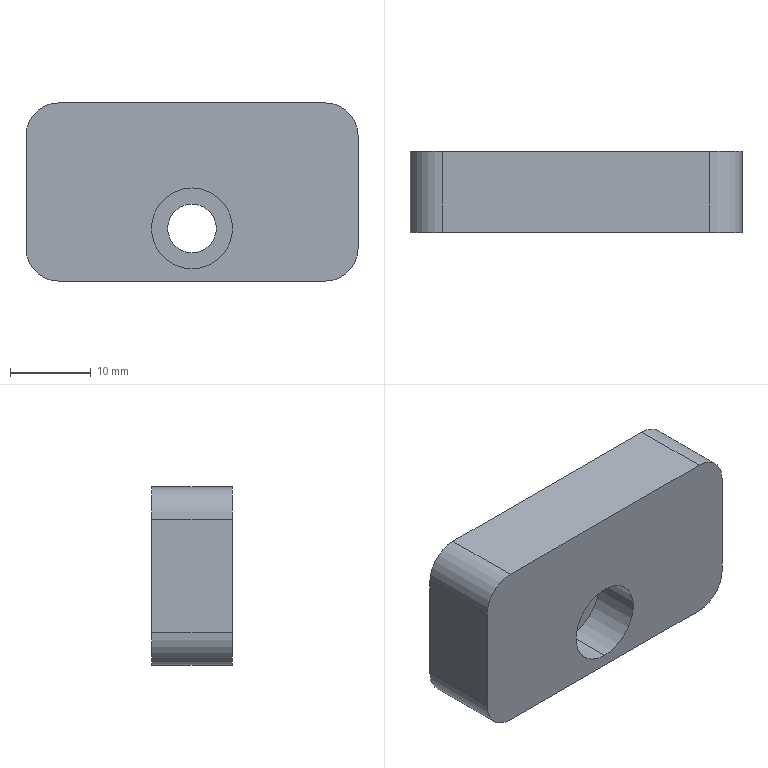Part | STEP file | 1 solid | 15 faces | box 41 x 10 x 22 mm | volume 8298 mm3 | cylinder 8 | plane 7 | commonest cylinder face diameters 8 x4 6 x2 10 x2
STEP:
#1=CARTESIAN_POINT('',(0.,0.,0.));
#2=DIRECTION('',(0.,0.,1.));
#3=DIRECTION('',(1.,0.,0.));
#4=AXIS2_PLACEMENT_3D('',#1,#2,#3);
#5=CARTESIAN_POINT('',(-118.59,-44.,195.714));
#6=VERTEX_POINT('',#5);
#7=CARTESIAN_POINT('',(-118.59,-40.,195.714));
#8=VERTEX_POINT('',#7);
#9=CARTESIAN_POINT('',(-118.59,-50.,195.714));
#10=DIRECTION('',(0.,1.,0.));
#11=VECTOR('',#10,1.);
#12=LINE('',#9,#11);
#13=CARTESIAN_POINT('',(-118.59,-50.,192.714));
#14=DIRECTION('',(0.,1.,0.));
#15=DIRECTION('',(0.,0.,1.));
#16=AXIS2_PLACEMENT_3D('',#13,#14,#15);
#17=CYLINDRICAL_SURFACE('',#16,3.);
#18=CARTESIAN_POINT('',(6.283,0.));
#19=DIRECTION('',(0.,1.));
#20=VECTOR('',#19,1.);
#21=LINE('',#18,#20);
#22=(GEOMETRIC_REPRESENTATION_CONTEXT(2)PARAMETRIC_REPRESENTATION_CONTEXT()REPRESENTATION_CONTEXT('',''));
#23=DEFINITIONAL_REPRESENTATION('',(#21),#22);
#24=PCURVE('',#17,#23);
#25=CARTESIAN_POINT('',(-118.59,-50.,192.714));
#26=DIRECTION('',(0.,1.,0.));
#27=DIRECTION('',(0.,0.,1.));
#28=AXIS2_PLACEMENT_3D('',#25,#26,#27);
#29=CYLINDRICAL_SURFACE('',#28,3.);
#30=CARTESIAN_POINT('',(0.,0.));
#31=DIRECTION('',(0.,1.));
#32=VECTOR('',#31,1.);
#33=LINE('',#30,#32);
#34=(GEOMETRIC_REPRESENTATION_CONTEXT(2)PARAMETRIC_REPRESENTATION_CONTEXT()REPRESENTATION_CONTEXT('',''));
#35=DEFINITIONAL_REPRESENTATION('',(#33),#34);
#36=PCURVE('',#29,#35);
#37=SURFACE_CURVE('',#12,(#24,#36),.PCURVE_S1.);
#38=EDGE_CURVE('',#6,#8,#37,.T.);
#39=ORIENTED_EDGE('',*,*,#38,.T.);
#40=CARTESIAN_POINT('',(-118.59,-40.,189.714));
#41=VERTEX_POINT('',#40);
#42=CARTESIAN_POINT('',(-118.59,-40.,192.714));
#43=DIRECTION('',(0.,-1.,0.));
#44=DIRECTION('',(0.,0.,-1.));
#45=AXIS2_PLACEMENT_3D('',#42,#43,#44);
#46=CIRCLE('',#45,3.);
#47=CARTESIAN_POINT('',(9.425,10.));
#48=DIRECTION('',(-1.,0.));
#49=VECTOR('',#48,1.);
#50=LINE('',#47,#49);
#51=(GEOMETRIC_REPRESENTATION_CONTEXT(2)PARAMETRIC_REPRESENTATION_CONTEXT()REPRESENTATION_CONTEXT('',''));
#52=DEFINITIONAL_REPRESENTATION('',(#50),#51);
#53=PCURVE('',#17,#52);
#54=CARTESIAN_POINT('',(-118.59,-40.,193.714));
#55=DIRECTION('',(0.,-1.,0.));
#56=DIRECTION('',(0.,0.,-1.));
#57=AXIS2_PLACEMENT_3D('',#54,#55,#56);
#58=PLANE('',#57);
#59=CARTESIAN_POINT('',(1.,0.));
#60=DIRECTION('',(1.,0.));
#61=AXIS2_PLACEMENT_2D('',#59,#60);
#62=CIRCLE('',#61,3.);
#63=(GEOMETRIC_REPRESENTATION_CONTEXT(2)PARAMETRIC_REPRESENTATION_CONTEXT()REPRESENTATION_CONTEXT('',''));
#64=DEFINITIONAL_REPRESENTATION('',(#62),#63);
#65=PCURVE('',#58,#64);
#66=SURFACE_CURVE('',#46,(#53,#65),.PCURVE_S1.);
#67=EDGE_CURVE('',#8,#41,#66,.T.);
#68=ORIENTED_EDGE('',*,*,#67,.T.);
#69=CARTESIAN_POINT('',(-118.59,-44.,189.714));
#70=VERTEX_POINT('',#69);
#71=CARTESIAN_POINT('',(-118.59,-50.,189.714));
#72=DIRECTION('',(0.,1.,0.));
#73=VECTOR('',#72,1.);
#74=LINE('',#71,#73);
#75=CARTESIAN_POINT('',(3.142,0.));
#76=DIRECTION('',(0.,1.));
#77=VECTOR('',#76,1.);
#78=LINE('',#75,#77);
#79=(GEOMETRIC_REPRESENTATION_CONTEXT(2)PARAMETRIC_REPRESENTATION_CONTEXT()REPRESENTATION_CONTEXT('',''));
#80=DEFINITIONAL_REPRESENTATION('',(#78),#79);
#81=PCURVE('',#17,#80);
#82=CARTESIAN_POINT('',(3.142,0.));
#83=DIRECTION('',(0.,1.));
#84=VECTOR('',#83,1.);
#85=LINE('',#82,#84);
#86=(GEOMETRIC_REPRESENTATION_CONTEXT(2)PARAMETRIC_REPRESENTATION_CONTEXT()REPRESENTATION_CONTEXT('',''));
#87=DEFINITIONAL_REPRESENTATION('',(#85),#86);
#88=PCURVE('',#29,#87);
#89=SURFACE_CURVE('',#74,(#81,#88),.PCURVE_S1.);
#90=EDGE_CURVE('',#70,#41,#89,.T.);
#91=ORIENTED_EDGE('',*,*,#90,.F.);
#92=CARTESIAN_POINT('',(-118.59,-44.,192.714));
#93=DIRECTION('',(0.,-1.,0.));
#94=DIRECTION('',(0.,0.,1.));
#95=AXIS2_PLACEMENT_3D('',#92,#93,#94);
#96=CIRCLE('',#95,3.);
#97=CARTESIAN_POINT('',(6.283,6.));
#98=DIRECTION('',(-1.,0.));
#99=VECTOR('',#98,1.);
#100=LINE('',#97,#99);
#101=(GEOMETRIC_REPRESENTATION_CONTEXT(2)PARAMETRIC_REPRESENTATION_CONTEXT()REPRESENTATION_CONTEXT('',''));
#102=DEFINITIONAL_REPRESENTATION('',(#100),#101);
#103=PCURVE('',#17,#102);
#104=CARTESIAN_POINT('',(-118.59,-44.,192.714));
#105=DIRECTION('',(0.,1.,0.));
#106=DIRECTION('',(0.,0.,1.));
#107=AXIS2_PLACEMENT_3D('',#104,#105,#106);
#108=PLANE('',#107);
#109=CARTESIAN_POINT('',(3.,0.));
#110=CARTESIAN_POINT('',(3.,-5.196));
#111=CARTESIAN_POINT('',(-1.5,-2.598));
#112=CARTESIAN_POINT('',(-6.,0.));
#113=CARTESIAN_POINT('',(-1.5,2.598));
#114=CARTESIAN_POINT('',(3.,5.196));
#115=CARTESIAN_POINT('',(3.,0.));
#116=(BOUNDED_CURVE()B_SPLINE_CURVE(2,(#109,#110,#111,#112,#113,#114,#115),.UNSPECIFIED.,.T.,.F.)B_SPLINE_CURVE_WITH_KNOTS((1,2,2,2,2,1),(-2.094,0.,2.094,4.189,6.283,8.378),.UNSPECIFIED.)CURVE()GEOMETRIC_REPRESENTATION_ITEM()RATIONAL_B_SPLINE_CURVE((1.,0.5,1.,0.5,1.,0.5,1.))REPRESENTATION_ITEM(''));
#117=(GEOMETRIC_REPRESENTATION_CONTEXT(2)PARAMETRIC_REPRESENTATION_CONTEXT()REPRESENTATION_CONTEXT('',''));
#118=DEFINITIONAL_REPRESENTATION('',(#116),#117);
#119=PCURVE('',#108,#118);
#120=SURFACE_CURVE('',#96,(#103,#119),.PCURVE_S1.);
#121=EDGE_CURVE('',#6,#70,#120,.T.);
#122=ORIENTED_EDGE('',*,*,#121,.F.);
#123=EDGE_LOOP('',(#39,#68,#91,#122));
#124=FACE_BOUND('',#123,.F.);
#125=ADVANCED_FACE('',(#124),#17,.F.);
#126=CARTESIAN_POINT('',(-118.59,-50.,197.714));
#127=VERTEX_POINT('',#126);
#128=CARTESIAN_POINT('',(-118.59,-44.,197.714));
#129=VERTEX_POINT('',#128);
#130=CARTESIAN_POINT('',(-118.59,-50.,197.714));
#131=DIRECTION('',(0.,1.,0.));
#132=VECTOR('',#131,1.);
#133=LINE('',#130,#132);
#134=CARTESIAN_POINT('',(-118.59,-50.,192.714));
#135=DIRECTION('',(0.,1.,0.));
#136=DIRECTION('',(0.,0.,1.));
#137=AXIS2_PLACEMENT_3D('',#134,#135,#136);
#138=CYLINDRICAL_SURFACE('',#137,5.);
#139=CARTESIAN_POINT('',(6.283,0.));
#140=DIRECTION('',(0.,1.));
#141=VECTOR('',#140,1.);
#142=LINE('',#139,#141);
#143=(GEOMETRIC_REPRESENTATION_CONTEXT(2)PARAMETRIC_REPRESENTATION_CONTEXT()REPRESENTATION_CONTEXT('',''));
#144=DEFINITIONAL_REPRESENTATION('',(#142),#143);
#145=PCURVE('',#138,#144);
#146=CARTESIAN_POINT('',(-118.59,-50.,192.714));
#147=DIRECTION('',(0.,1.,0.));
#148=DIRECTION('',(0.,0.,1.));
#149=AXIS2_PLACEMENT_3D('',#146,#147,#148);
#150=CYLINDRICAL_SURFACE('',#149,5.);
#151=CARTESIAN_POINT('',(0.,0.));
#152=DIRECTION('',(0.,1.));
#153=VECTOR('',#152,1.);
#154=LINE('',#151,#153);
#155=(GEOMETRIC_REPRESENTATION_CONTEXT(2)PARAMETRIC_REPRESENTATION_CONTEXT()REPRESENTATION_CONTEXT('',''));
#156=DEFINITIONAL_REPRESENTATION('',(#154),#155);
#157=PCURVE('',#150,#156);
#158=SURFACE_CURVE('',#133,(#145,#157),.PCURVE_S1.);
#159=EDGE_CURVE('',#127,#129,#158,.T.);
#160=ORIENTED_EDGE('',*,*,#159,.T.);
#161=CARTESIAN_POINT('',(-118.59,-44.,187.714));
#162=VERTEX_POINT('',#161);
#163=CARTESIAN_POINT('',(-118.59,-44.,192.714));
#164=DIRECTION('',(0.,-1.,0.));
#165=DIRECTION('',(0.,0.,-1.));
#166=AXIS2_PLACEMENT_3D('',#163,#164,#165);
#167=CIRCLE('',#166,5.);
#168=CARTESIAN_POINT('',(9.425,6.));
#169=DIRECTION('',(-1.,0.));
#170=VECTOR('',#169,1.);
#171=LINE('',#168,#170);
#172=(GEOMETRIC_REPRESENTATION_CONTEXT(2)PARAMETRIC_REPRESENTATION_CONTEXT()REPRESENTATION_CONTEXT('',''));
#173=DEFINITIONAL_REPRESENTATION('',(#171),#172);
#174=PCURVE('',#138,#173);
#175=CARTESIAN_POINT('',(-5.,0.));
#176=CARTESIAN_POINT('',(-5.,8.66));
#177=CARTESIAN_POINT('',(2.5,4.33));
#178=CARTESIAN_POINT('',(10.,0.));
#179=CARTESIAN_POINT('',(2.5,-4.33));
#180=CARTESIAN_POINT('',(-5.,-8.66));
#181=CARTESIAN_POINT('',(-5.,0.));
#182=(BOUNDED_CURVE()B_SPLINE_CURVE(2,(#175,#176,#177,#178,#179,#180,#181),.UNSPECIFIED.,.T.,.F.)B_SPLINE_CURVE_WITH_KNOTS((1,2,2,2,2,1),(-2.094,0.,2.094,4.189,6.283,8.378),.UNSPECIFIED.)CURVE()GEOMETRIC_REPRESENTATION_ITEM()RATIONAL_B_SPLINE_CURVE((1.,0.5,1.,0.5,1.,0.5,1.))REPRESENTATION_ITEM(''));
#183=(GEOMETRIC_REPRESENTATION_CONTEXT(2)PARAMETRIC_REPRESENTATION_CONTEXT()REPRESENTATION_CONTEXT('',''));
#184=DEFINITIONAL_REPRESENTATION('',(#182),#183);
#185=PCURVE('',#108,#184);
#186=SURFACE_CURVE('',#167,(#174,#185),.PCURVE_S1.);
#187=EDGE_CURVE('',#129,#162,#186,.T.);
#188=ORIENTED_EDGE('',*,*,#187,.T.);
#189=CARTESIAN_POINT('',(-118.59,-50.,187.714));
#190=VERTEX_POINT('',#189);
#191=CARTESIAN_POINT('',(-118.59,-50.,187.714));
#192=DIRECTION('',(0.,1.,0.));
#193=VECTOR('',#192,1.);
#194=LINE('',#191,#193);
#195=CARTESIAN_POINT('',(3.142,0.));
#196=DIRECTION('',(0.,1.));
#197=VECTOR('',#196,1.);
#198=LINE('',#195,#197);
#199=(GEOMETRIC_REPRESENTATION_CONTEXT(2)PARAMETRIC_REPRESENTATION_CONTEXT()REPRESENTATION_CONTEXT('',''));
#200=DEFINITIONAL_REPRESENTATION('',(#198),#199);
#201=PCURVE('',#138,#200);
#202=CARTESIAN_POINT('',(3.142,0.));
#203=DIRECTION('',(0.,1.));
#204=VECTOR('',#203,1.);
#205=LINE('',#202,#204);
#206=(GEOMETRIC_REPRESENTATION_CONTEXT(2)PARAMETRIC_REPRESENTATION_CONTEXT()REPRESENTATION_CONTEXT('',''));
#207=DEFINITIONAL_REPRESENTATION('',(#205),#206);
#208=PCURVE('',#150,#207);
#209=SURFACE_CURVE('',#194,(#201,#208),.PCURVE_S1.);
#210=EDGE_CURVE('',#190,#162,#209,.T.);
#211=ORIENTED_EDGE('',*,*,#210,.F.);
#212=CARTESIAN_POINT('',(-118.59,-50.,192.714));
#213=DIRECTION('',(0.,1.,0.));
#214=DIRECTION('',(0.,0.,1.));
#215=AXIS2_PLACEMENT_3D('',#212,#213,#214);
#216=CIRCLE('',#215,5.);
#217=CARTESIAN_POINT('',(0.,0.));
#218=DIRECTION('',(1.,0.));
#219=VECTOR('',#218,1.);
#220=LINE('',#217,#219);
#221=(GEOMETRIC_REPRESENTATION_CONTEXT(2)PARAMETRIC_REPRESENTATION_CONTEXT()REPRESENTATION_CONTEXT('',''));
#222=DEFINITIONAL_REPRESENTATION('',(#220),#221);
#223=PCURVE('',#138,#222);
#224=CARTESIAN_POINT('',(-118.59,-50.,189.963));
#225=DIRECTION('',(0.,-1.,0.));
#226=DIRECTION('',(0.,0.,-1.));
#227=AXIS2_PLACEMENT_3D('',#224,#225,#226);
#228=PLANE('',#227);
#229=CARTESIAN_POINT('',(-7.751,0.));
#230=CARTESIAN_POINT('',(-7.751,8.66));
#231=CARTESIAN_POINT('',(-0.2512,4.33));
#232=CARTESIAN_POINT('',(7.249,0.));
#233=CARTESIAN_POINT('',(-0.2512,-4.33));
#234=CARTESIAN_POINT('',(-7.751,-8.66));
#235=CARTESIAN_POINT('',(-7.751,0.));
#236=(BOUNDED_CURVE()B_SPLINE_CURVE(2,(#229,#230,#231,#232,#233,#234,#235),.UNSPECIFIED.,.T.,.F.)B_SPLINE_CURVE_WITH_KNOTS((1,2,2,2,2,1),(-2.094,0.,2.094,4.189,6.283,8.378),.UNSPECIFIED.)CURVE()GEOMETRIC_REPRESENTATION_ITEM()RATIONAL_B_SPLINE_CURVE((1.,0.5,1.,0.5,1.,0.5,1.))REPRESENTATION_ITEM(''));
#237=(GEOMETRIC_REPRESENTATION_CONTEXT(2)PARAMETRIC_REPRESENTATION_CONTEXT()REPRESENTATION_CONTEXT('',''));
#238=DEFINITIONAL_REPRESENTATION('',(#236),#237);
#239=PCURVE('',#228,#238);
#240=SURFACE_CURVE('',#216,(#223,#239),.PCURVE_S1.);
#241=EDGE_CURVE('',#190,#127,#240,.T.);
#242=ORIENTED_EDGE('',*,*,#241,.T.);
#243=EDGE_LOOP('',(#160,#188,#211,#242));
#244=FACE_BOUND('',#243,.F.);
#245=ADVANCED_FACE('',(#244),#138,.F.);
#246=CARTESIAN_POINT('',(-102.09,-50.,208.214));
#247=VERTEX_POINT('',#246);
#248=CARTESIAN_POINT('',(-135.09,-50.,208.214));
#249=VERTEX_POINT('',#248);
#250=CARTESIAN_POINT('',(-118.59,-50.,208.214));
#251=DIRECTION('',(-1.,0.,0.));
#252=VECTOR('',#251,1.);
#253=LINE('',#250,#252);
#254=CARTESIAN_POINT('',(-18.251,0.));
#255=DIRECTION('',(0.,-1.));
#256=VECTOR('',#255,1.);
#257=LINE('',#254,#256);
#258=(GEOMETRIC_REPRESENTATION_CONTEXT(2)PARAMETRIC_REPRESENTATION_CONTEXT()REPRESENTATION_CONTEXT('',''));
#259=DEFINITIONAL_REPRESENTATION('',(#257),#258);
#260=PCURVE('',#228,#259);
#261=CARTESIAN_POINT('',(-98.09,-40.,208.214));
#262=DIRECTION('',(0.,0.,1.));
#263=DIRECTION('',(1.,0.,0.));
#264=AXIS2_PLACEMENT_3D('',#261,#262,#263);
#265=PLANE('',#264);
#266=CARTESIAN_POINT('',(-20.5,-10.));
#267=DIRECTION('',(-1.,0.));
#268=VECTOR('',#267,1.);
#269=LINE('',#266,#268);
#270=(GEOMETRIC_REPRESENTATION_CONTEXT(2)PARAMETRIC_REPRESENTATION_CONTEXT()REPRESENTATION_CONTEXT('',''));
#271=DEFINITIONAL_REPRESENTATION('',(#269),#270);
#272=PCURVE('',#265,#271);
#273=SURFACE_CURVE('',#253,(#260,#272),.PCURVE_S1.);
#274=EDGE_CURVE('',#247,#249,#273,.T.);
#275=ORIENTED_EDGE('',*,*,#274,.T.);
#276=CARTESIAN_POINT('',(-139.09,-50.,204.214));
#277=VERTEX_POINT('',#276);
#278=CARTESIAN_POINT('',(-135.09,-50.,204.214));
#279=DIRECTION('',(0.,-1.,0.));
#280=DIRECTION('',(0.,0.,-1.));
#281=AXIS2_PLACEMENT_3D('',#278,#279,#280);
#282=CIRCLE('',#281,4.);
#283=CARTESIAN_POINT('',(-14.251,-16.5));
#284=DIRECTION('',(1.,0.));
#285=AXIS2_PLACEMENT_2D('',#283,#284);
#286=CIRCLE('',#285,4.);
#287=(GEOMETRIC_REPRESENTATION_CONTEXT(2)PARAMETRIC_REPRESENTATION_CONTEXT()REPRESENTATION_CONTEXT('',''));
#288=DEFINITIONAL_REPRESENTATION('',(#286),#287);
#289=PCURVE('',#228,#288);
#290=CARTESIAN_POINT('',(-135.09,-50.,204.214));
#291=DIRECTION('',(0.,-1.,0.));
#292=DIRECTION('',(0.,0.,-1.));
#293=AXIS2_PLACEMENT_3D('',#290,#291,#292);
#294=CYLINDRICAL_SURFACE('',#293,4.);
#295=CARTESIAN_POINT('',(0.,0.));
#296=DIRECTION('',(1.,0.));
#297=VECTOR('',#296,1.);
#298=LINE('',#295,#297);
#299=(GEOMETRIC_REPRESENTATION_CONTEXT(2)PARAMETRIC_REPRESENTATION_CONTEXT()REPRESENTATION_CONTEXT('',''));
#300=DEFINITIONAL_REPRESENTATION('',(#298),#299);
#301=PCURVE('',#294,#300);
#302=SURFACE_CURVE('',#282,(#289,#301),.PCURVE_S1.);
#303=EDGE_CURVE('',#249,#277,#302,.T.);
#304=ORIENTED_EDGE('',*,*,#303,.T.);
#305=CARTESIAN_POINT('',(-139.09,-50.,190.214));
#306=VERTEX_POINT('',#305);
#307=CARTESIAN_POINT('',(-139.09,-50.,189.963));
#308=DIRECTION('',(0.,0.,1.));
#309=VECTOR('',#308,1.);
#310=LINE('',#307,#309);
#311=CARTESIAN_POINT('',(0.,-20.5));
#312=DIRECTION('',(-1.,0.));
#313=VECTOR('',#312,1.);
#314=LINE('',#311,#313);
#315=(GEOMETRIC_REPRESENTATION_CONTEXT(2)PARAMETRIC_REPRESENTATION_CONTEXT()REPRESENTATION_CONTEXT('',''));
#316=DEFINITIONAL_REPRESENTATION('',(#314),#315);
#317=PCURVE('',#228,#316);
#318=CARTESIAN_POINT('',(-139.09,-50.,202.465));
#319=DIRECTION('',(1.,0.,0.));
#320=DIRECTION('',(0.,0.,-1.));
#321=AXIS2_PLACEMENT_3D('',#318,#319,#320);
#322=PLANE('',#321);
#323=CARTESIAN_POINT('',(12.502,0.));
#324=DIRECTION('',(-1.,0.));
#325=VECTOR('',#324,1.);
#326=LINE('',#323,#325);
#327=(GEOMETRIC_REPRESENTATION_CONTEXT(2)PARAMETRIC_REPRESENTATION_CONTEXT()REPRESENTATION_CONTEXT('',''));
#328=DEFINITIONAL_REPRESENTATION('',(#326),#327);
#329=PCURVE('',#322,#328);
#330=SURFACE_CURVE('',#310,(#317,#329),.PCURVE_S1.);
#331=EDGE_CURVE('',#306,#277,#330,.T.);
#332=ORIENTED_EDGE('',*,*,#331,.F.);
#333=CARTESIAN_POINT('',(-135.09,-50.,186.214));
#334=VERTEX_POINT('',#333);
#335=CARTESIAN_POINT('',(-135.09,-50.,190.214));
#336=DIRECTION('',(0.,-1.,0.));
#337=DIRECTION('',(0.,0.,-1.));
#338=AXIS2_PLACEMENT_3D('',#335,#336,#337);
#339=CIRCLE('',#338,4.);
#340=CARTESIAN_POINT('',(-0.2512,-16.5));
#341=DIRECTION('',(1.,0.));
#342=AXIS2_PLACEMENT_2D('',#340,#341);
#343=CIRCLE('',#342,4.);
#344=(GEOMETRIC_REPRESENTATION_CONTEXT(2)PARAMETRIC_REPRESENTATION_CONTEXT()REPRESENTATION_CONTEXT('',''));
#345=DEFINITIONAL_REPRESENTATION('',(#343),#344);
#346=PCURVE('',#228,#345);
#347=CARTESIAN_POINT('',(-135.09,-50.,190.214));
#348=DIRECTION('',(0.,-1.,0.));
#349=DIRECTION('',(0.,0.,-1.));
#350=AXIS2_PLACEMENT_3D('',#347,#348,#349);
#351=CYLINDRICAL_SURFACE('',#350,4.);
#352=CARTESIAN_POINT('',(0.,0.));
#353=DIRECTION('',(1.,0.));
#354=VECTOR('',#353,1.);
#355=LINE('',#352,#354);
#356=(GEOMETRIC_REPRESENTATION_CONTEXT(2)PARAMETRIC_REPRESENTATION_CONTEXT()REPRESENTATION_CONTEXT('',''));
#357=DEFINITIONAL_REPRESENTATION('',(#355),#356);
#358=PCURVE('',#351,#357);
#359=SURFACE_CURVE('',#339,(#346,#358),.PCURVE_S1.);
#360=EDGE_CURVE('',#306,#334,#359,.T.);
#361=ORIENTED_EDGE('',*,*,#360,.T.);
#362=CARTESIAN_POINT('',(-102.09,-50.,186.214));
#363=VERTEX_POINT('',#362);
#364=CARTESIAN_POINT('',(-118.59,-50.,186.214));
#365=DIRECTION('',(-1.,0.,0.));
#366=VECTOR('',#365,1.);
#367=LINE('',#364,#366);
#368=CARTESIAN_POINT('',(3.749,0.));
#369=DIRECTION('',(0.,-1.));
#370=VECTOR('',#369,1.);
#371=LINE('',#368,#370);
#372=(GEOMETRIC_REPRESENTATION_CONTEXT(2)PARAMETRIC_REPRESENTATION_CONTEXT()REPRESENTATION_CONTEXT('',''));
#373=DEFINITIONAL_REPRESENTATION('',(#371),#372);
#374=PCURVE('',#228,#373);
#375=CARTESIAN_POINT('',(-98.09,-40.,186.214));
#376=DIRECTION('',(0.,0.,1.));
#377=DIRECTION('',(1.,0.,0.));
#378=AXIS2_PLACEMENT_3D('',#375,#376,#377);
#379=PLANE('',#378);
#380=CARTESIAN_POINT('',(-20.5,-10.));
#381=DIRECTION('',(-1.,0.));
#382=VECTOR('',#381,1.);
#383=LINE('',#380,#382);
#384=(GEOMETRIC_REPRESENTATION_CONTEXT(2)PARAMETRIC_REPRESENTATION_CONTEXT()REPRESENTATION_CONTEXT('',''));
#385=DEFINITIONAL_REPRESENTATION('',(#383),#384);
#386=PCURVE('',#379,#385);
#387=SURFACE_CURVE('',#367,(#374,#386),.PCURVE_S1.);
#388=EDGE_CURVE('',#363,#334,#387,.T.);
#389=ORIENTED_EDGE('',*,*,#388,.F.);
#390=CARTESIAN_POINT('',(-98.09,-50.,190.214));
#391=VERTEX_POINT('',#390);
#392=CARTESIAN_POINT('',(-102.09,-50.,190.214));
#393=DIRECTION('',(0.,-1.,0.));
#394=DIRECTION('',(0.,0.,-1.));
#395=AXIS2_PLACEMENT_3D('',#392,#393,#394);
#396=CIRCLE('',#395,4.);
#397=CARTESIAN_POINT('',(-0.2512,16.5));
#398=DIRECTION('',(1.,0.));
#399=AXIS2_PLACEMENT_2D('',#397,#398);
#400=CIRCLE('',#399,4.);
#401=(GEOMETRIC_REPRESENTATION_CONTEXT(2)PARAMETRIC_REPRESENTATION_CONTEXT()REPRESENTATION_CONTEXT('',''));
#402=DEFINITIONAL_REPRESENTATION('',(#400),#401);
#403=PCURVE('',#228,#402);
#404=CARTESIAN_POINT('',(-102.09,-40.,190.214));
#405=DIRECTION('',(0.,1.,0.));
#406=DIRECTION('',(0.,0.,1.));
#407=AXIS2_PLACEMENT_3D('',#404,#405,#406);
#408=CYLINDRICAL_SURFACE('',#407,4.);
#409=CARTESIAN_POINT('',(3.142,-10.));
#410=DIRECTION('',(-1.,0.));
#411=VECTOR('',#410,1.);
#412=LINE('',#409,#411);
#413=(GEOMETRIC_REPRESENTATION_CONTEXT(2)PARAMETRIC_REPRESENTATION_CONTEXT()REPRESENTATION_CONTEXT('',''));
#414=DEFINITIONAL_REPRESENTATION('',(#412),#413);
#415=PCURVE('',#408,#414);
#416=SURFACE_CURVE('',#396,(#403,#415),.PCURVE_S1.);
#417=EDGE_CURVE('',#363,#391,#416,.T.);
#418=ORIENTED_EDGE('',*,*,#417,.T.);
#419=CARTESIAN_POINT('',(-98.09,-50.,204.214));
#420=VERTEX_POINT('',#419);
#421=CARTESIAN_POINT('',(-98.09,-50.,189.963));
#422=DIRECTION('',(0.,0.,1.));
#423=VECTOR('',#422,1.);
#424=LINE('',#421,#423);
#425=CARTESIAN_POINT('',(0.,20.5));
#426=DIRECTION('',(-1.,0.));
#427=VECTOR('',#426,1.);
#428=LINE('',#425,#427);
#429=(GEOMETRIC_REPRESENTATION_CONTEXT(2)PARAMETRIC_REPRESENTATION_CONTEXT()REPRESENTATION_CONTEXT('',''));
#430=DEFINITIONAL_REPRESENTATION('',(#428),#429);
#431=PCURVE('',#228,#430);
#432=CARTESIAN_POINT('',(-98.09,-50.,202.465));
#433=DIRECTION('',(1.,0.,0.));
#434=DIRECTION('',(0.,0.,-1.));
#435=AXIS2_PLACEMENT_3D('',#432,#433,#434);
#436=PLANE('',#435);
#437=CARTESIAN_POINT('',(12.502,0.));
#438=DIRECTION('',(-1.,0.));
#439=VECTOR('',#438,1.);
#440=LINE('',#437,#439);
#441=(GEOMETRIC_REPRESENTATION_CONTEXT(2)PARAMETRIC_REPRESENTATION_CONTEXT()REPRESENTATION_CONTEXT('',''));
#442=DEFINITIONAL_REPRESENTATION('',(#440),#441);
#443=PCURVE('',#436,#442);
#444=SURFACE_CURVE('',#424,(#431,#443),.PCURVE_S1.);
#445=EDGE_CURVE('',#391,#420,#444,.T.);
#446=ORIENTED_EDGE('',*,*,#445,.T.);
#447=CARTESIAN_POINT('',(-102.09,-50.,204.214));
#448=DIRECTION('',(0.,-1.,0.));
#449=DIRECTION('',(0.,0.,-1.));
#450=AXIS2_PLACEMENT_3D('',#447,#448,#449);
#451=CIRCLE('',#450,4.);
#452=CARTESIAN_POINT('',(-14.251,16.5));
#453=DIRECTION('',(1.,0.));
#454=AXIS2_PLACEMENT_2D('',#452,#453);
#455=CIRCLE('',#454,4.);
#456=(GEOMETRIC_REPRESENTATION_CONTEXT(2)PARAMETRIC_REPRESENTATION_CONTEXT()REPRESENTATION_CONTEXT('',''));
#457=DEFINITIONAL_REPRESENTATION('',(#455),#456);
#458=PCURVE('',#228,#457);
#459=CARTESIAN_POINT('',(-102.09,-40.,204.214));
#460=DIRECTION('',(0.,1.,0.));
#461=DIRECTION('',(0.,0.,1.));
#462=AXIS2_PLACEMENT_3D('',#459,#460,#461);
#463=CYLINDRICAL_SURFACE('',#462,4.);
#464=CARTESIAN_POINT('',(3.142,-10.));
#465=DIRECTION('',(-1.,0.));
#466=VECTOR('',#465,1.);
#467=LINE('',#464,#466);
#468=(GEOMETRIC_REPRESENTATION_CONTEXT(2)PARAMETRIC_REPRESENTATION_CONTEXT()REPRESENTATION_CONTEXT('',''));
#469=DEFINITIONAL_REPRESENTATION('',(#467),#468);
#470=PCURVE('',#463,#469);
#471=SURFACE_CURVE('',#451,(#458,#470),.PCURVE_S1.);
#472=EDGE_CURVE('',#420,#247,#471,.T.);
#473=ORIENTED_EDGE('',*,*,#472,.T.);
#474=EDGE_LOOP('',(#275,#304,#332,#361,#389,#418,#446,#473));
#475=FACE_BOUND('',#474,.T.);
#476=CARTESIAN_POINT('',(-118.59,-50.,192.714));
#477=DIRECTION('',(0.,1.,0.));
#478=DIRECTION('',(0.,0.,1.));
#479=AXIS2_PLACEMENT_3D('',#476,#477,#478);
#480=CIRCLE('',#479,5.);
#481=CARTESIAN_POINT('',(-7.751,0.));
#482=CARTESIAN_POINT('',(-7.751,8.66));
#483=CARTESIAN_POINT('',(-0.2512,4.33));
#484=CARTESIAN_POINT('',(7.249,0.));
#485=CARTESIAN_POINT('',(-0.2512,-4.33));
#486=CARTESIAN_POINT('',(-7.751,-8.66));
#487=CARTESIAN_POINT('',(-7.751,0.));
#488=(BOUNDED_CURVE()B_SPLINE_CURVE(2,(#481,#482,#483,#484,#485,#486,#487),.UNSPECIFIED.,.T.,.F.)B_SPLINE_CURVE_WITH_KNOTS((1,2,2,2,2,1),(-2.094,0.,2.094,4.189,6.283,8.378),.UNSPECIFIED.)CURVE()GEOMETRIC_REPRESENTATION_ITEM()RATIONAL_B_SPLINE_CURVE((1.,0.5,1.,0.5,1.,0.5,1.))REPRESENTATION_ITEM(''));
#489=(GEOMETRIC_REPRESENTATION_CONTEXT(2)PARAMETRIC_REPRESENTATION_CONTEXT()REPRESENTATION_CONTEXT('',''));
#490=DEFINITIONAL_REPRESENTATION('',(#488),#489);
#491=PCURVE('',#228,#490);
#492=CARTESIAN_POINT('',(0.,0.));
#493=DIRECTION('',(1.,0.));
#494=VECTOR('',#493,1.);
#495=LINE('',#492,#494);
#496=(GEOMETRIC_REPRESENTATION_CONTEXT(2)PARAMETRIC_REPRESENTATION_CONTEXT()REPRESENTATION_CONTEXT('',''));
#497=DEFINITIONAL_REPRESENTATION('',(#495),#496);
#498=PCURVE('',#150,#497);
#499=SURFACE_CURVE('',#480,(#491,#498),.PCURVE_S1.);
#500=EDGE_CURVE('',#127,#190,#499,.T.);
#501=ORIENTED_EDGE('',*,*,#500,.T.);
#502=ORIENTED_EDGE('',*,*,#241,.T.);
#503=EDGE_LOOP('',(#501,#502));
#504=FACE_BOUND('',#503,.T.);
#505=ADVANCED_FACE('',(#475,#504),#228,.T.);
#506=CARTESIAN_POINT('',(-102.09,-40.,208.214));
#507=VERTEX_POINT('',#506);
#508=CARTESIAN_POINT('',(-135.09,-40.,208.214));
#509=VERTEX_POINT('',#508);
#510=CARTESIAN_POINT('',(-118.59,-40.,208.214));
#511=DIRECTION('',(-1.,0.,0.));
#512=VECTOR('',#511,1.);
#513=LINE('',#510,#512);
#514=CARTESIAN_POINT('',(-20.5,0.));
#515=DIRECTION('',(-1.,0.));
#516=VECTOR('',#515,1.);
#517=LINE('',#514,#516);
#518=(GEOMETRIC_REPRESENTATION_CONTEXT(2)PARAMETRIC_REPRESENTATION_CONTEXT()REPRESENTATION_CONTEXT('',''));
#519=DEFINITIONAL_REPRESENTATION('',(#517),#518);
#520=PCURVE('',#265,#519);
#521=CARTESIAN_POINT('',(-14.5,0.));
#522=DIRECTION('',(0.,-1.));
#523=VECTOR('',#522,1.);
#524=LINE('',#521,#523);
#525=(GEOMETRIC_REPRESENTATION_CONTEXT(2)PARAMETRIC_REPRESENTATION_CONTEXT()REPRESENTATION_CONTEXT('',''));
#526=DEFINITIONAL_REPRESENTATION('',(#524),#525);
#527=PCURVE('',#58,#526);
#528=SURFACE_CURVE('',#513,(#520,#527),.PCURVE_S1.);
#529=EDGE_CURVE('',#507,#509,#528,.T.);
#530=ORIENTED_EDGE('',*,*,#529,.T.);
#531=CARTESIAN_POINT('',(-135.09,-50.,208.214));
#532=DIRECTION('',(0.,-1.,0.));
#533=VECTOR('',#532,1.);
#534=LINE('',#531,#533);
#535=CARTESIAN_POINT('',(-37.,-10.));
#536=DIRECTION('',(0.,-1.));
#537=VECTOR('',#536,1.);
#538=LINE('',#535,#537);
#539=(GEOMETRIC_REPRESENTATION_CONTEXT(2)PARAMETRIC_REPRESENTATION_CONTEXT()REPRESENTATION_CONTEXT('',''));
#540=DEFINITIONAL_REPRESENTATION('',(#538),#539);
#541=PCURVE('',#265,#540);
#542=CARTESIAN_POINT('',(3.142,0.));
#543=DIRECTION('',(0.,1.));
#544=VECTOR('',#543,1.);
#545=LINE('',#542,#544);
#546=(GEOMETRIC_REPRESENTATION_CONTEXT(2)PARAMETRIC_REPRESENTATION_CONTEXT()REPRESENTATION_CONTEXT('',''));
#547=DEFINITIONAL_REPRESENTATION('',(#545),#546);
#548=PCURVE('',#294,#547);
#549=SURFACE_CURVE('',#534,(#541,#548),.PCURVE_S1.);
#550=EDGE_CURVE('',#509,#249,#549,.T.);
#551=ORIENTED_EDGE('',*,*,#550,.T.);
#552=ORIENTED_EDGE('',*,*,#274,.F.);
#553=CARTESIAN_POINT('',(-102.09,-40.,208.214));
#554=DIRECTION('',(0.,1.,0.));
#555=VECTOR('',#554,1.);
#556=LINE('',#553,#555);
#557=CARTESIAN_POINT('',(-4.,0.));
#558=DIRECTION('',(0.,1.));
#559=VECTOR('',#558,1.);
#560=LINE('',#557,#559);
#561=(GEOMETRIC_REPRESENTATION_CONTEXT(2)PARAMETRIC_REPRESENTATION_CONTEXT()REPRESENTATION_CONTEXT('',''));
#562=DEFINITIONAL_REPRESENTATION('',(#560),#561);
#563=PCURVE('',#265,#562);
#564=CARTESIAN_POINT('',(0.,0.));
#565=DIRECTION('',(0.,1.));
#566=VECTOR('',#565,1.);
#567=LINE('',#564,#566);
#568=(GEOMETRIC_REPRESENTATION_CONTEXT(2)PARAMETRIC_REPRESENTATION_CONTEXT()REPRESENTATION_CONTEXT('',''));
#569=DEFINITIONAL_REPRESENTATION('',(#567),#568);
#570=PCURVE('',#463,#569);
#571=SURFACE_CURVE('',#556,(#563,#570),.PCURVE_S1.);
#572=EDGE_CURVE('',#247,#507,#571,.T.);
#573=ORIENTED_EDGE('',*,*,#572,.T.);
#574=EDGE_LOOP('',(#530,#551,#552,#573));
#575=FACE_BOUND('',#574,.T.);
#576=ADVANCED_FACE('',(#575),#265,.T.);
#577=ORIENTED_EDGE('',*,*,#331,.T.);
#578=CARTESIAN_POINT('',(-139.09,-40.,204.214));
#579=VERTEX_POINT('',#578);
#580=CARTESIAN_POINT('',(-139.09,-40.,204.214));
#581=DIRECTION('',(0.,1.,0.));
#582=VECTOR('',#581,1.);
#583=LINE('',#580,#582);
#584=CARTESIAN_POINT('',(-1.749,10.));
#585=DIRECTION('',(0.,1.));
#586=VECTOR('',#585,1.);
#587=LINE('',#584,#586);
#588=(GEOMETRIC_REPRESENTATION_CONTEXT(2)PARAMETRIC_REPRESENTATION_CONTEXT()REPRESENTATION_CONTEXT('',''));
#589=DEFINITIONAL_REPRESENTATION('',(#587),#588);
#590=PCURVE('',#322,#589);
#591=CARTESIAN_POINT('',(4.712,-10.));
#592=DIRECTION('',(0.,-1.));
#593=VECTOR('',#592,1.);
#594=LINE('',#591,#593);
#595=(GEOMETRIC_REPRESENTATION_CONTEXT(2)PARAMETRIC_REPRESENTATION_CONTEXT()REPRESENTATION_CONTEXT('',''));
#596=DEFINITIONAL_REPRESENTATION('',(#594),#595);
#597=PCURVE('',#294,#596);
#598=SURFACE_CURVE('',#583,(#590,#597),.PCURVE_S1.);
#599=EDGE_CURVE('',#277,#579,#598,.T.);
#600=ORIENTED_EDGE('',*,*,#599,.T.);
#601=CARTESIAN_POINT('',(-139.09,-40.,190.214));
#602=VERTEX_POINT('',#601);
#603=CARTESIAN_POINT('',(-139.09,-40.,193.714));
#604=DIRECTION('',(0.,0.,1.));
#605=VECTOR('',#604,1.);
#606=LINE('',#603,#605);
#607=CARTESIAN_POINT('',(8.751,10.));
#608=DIRECTION('',(-1.,0.));
#609=VECTOR('',#608,1.);
#610=LINE('',#607,#609);
#611=(GEOMETRIC_REPRESENTATION_CONTEXT(2)PARAMETRIC_REPRESENTATION_CONTEXT()REPRESENTATION_CONTEXT('',''));
#612=DEFINITIONAL_REPRESENTATION('',(#610),#611);
#613=PCURVE('',#322,#612);
#614=CARTESIAN_POINT('',(0.,-20.5));
#615=DIRECTION('',(-1.,0.));
#616=VECTOR('',#615,1.);
#617=LINE('',#614,#616);
#618=(GEOMETRIC_REPRESENTATION_CONTEXT(2)PARAMETRIC_REPRESENTATION_CONTEXT()REPRESENTATION_CONTEXT('',''));
#619=DEFINITIONAL_REPRESENTATION('',(#617),#618);
#620=PCURVE('',#58,#619);
#621=SURFACE_CURVE('',#606,(#613,#620),.PCURVE_S1.);
#622=EDGE_CURVE('',#602,#579,#621,.T.);
#623=ORIENTED_EDGE('',*,*,#622,.F.);
#624=CARTESIAN_POINT('',(-139.09,-50.,190.214));
#625=DIRECTION('',(0.,-1.,0.));
#626=VECTOR('',#625,1.);
#627=LINE('',#624,#626);
#628=CARTESIAN_POINT('',(12.251,0.));
#629=DIRECTION('',(0.,-1.));
#630=VECTOR('',#629,1.);
#631=LINE('',#628,#630);
#632=(GEOMETRIC_REPRESENTATION_CONTEXT(2)PARAMETRIC_REPRESENTATION_CONTEXT()REPRESENTATION_CONTEXT('',''));
#633=DEFINITIONAL_REPRESENTATION('',(#631),#632);
#634=PCURVE('',#322,#633);
#635=CARTESIAN_POINT('',(4.712,0.));
#636=DIRECTION('',(0.,1.));
#637=VECTOR('',#636,1.);
#638=LINE('',#635,#637);
#639=(GEOMETRIC_REPRESENTATION_CONTEXT(2)PARAMETRIC_REPRESENTATION_CONTEXT()REPRESENTATION_CONTEXT('',''));
#640=DEFINITIONAL_REPRESENTATION('',(#638),#639);
#641=PCURVE('',#351,#640);
#642=SURFACE_CURVE('',#627,(#634,#641),.PCURVE_S1.);
#643=EDGE_CURVE('',#602,#306,#642,.T.);
#644=ORIENTED_EDGE('',*,*,#643,.T.);
#645=EDGE_LOOP('',(#577,#600,#623,#644));
#646=FACE_BOUND('',#645,.T.);
#647=ADVANCED_FACE('',(#646),#322,.F.);
#648=ORIENTED_EDGE('',*,*,#67,.T.);
#649=CARTESIAN_POINT('',(-118.59,-40.,192.714));
#650=DIRECTION('',(0.,-1.,0.));
#651=DIRECTION('',(0.,0.,-1.));
#652=AXIS2_PLACEMENT_3D('',#649,#650,#651);
#653=CIRCLE('',#652,3.);
#654=CARTESIAN_POINT('',(1.,0.));
#655=DIRECTION('',(1.,0.));
#656=AXIS2_PLACEMENT_2D('',#654,#655);
#657=CIRCLE('',#656,3.);
#658=(GEOMETRIC_REPRESENTATION_CONTEXT(2)PARAMETRIC_REPRESENTATION_CONTEXT()REPRESENTATION_CONTEXT('',''));
#659=DEFINITIONAL_REPRESENTATION('',(#657),#658);
#660=PCURVE('',#58,#659);
#661=CARTESIAN_POINT('',(3.142,10.));
#662=DIRECTION('',(-1.,0.));
#663=VECTOR('',#662,1.);
#664=LINE('',#661,#663);
#665=(GEOMETRIC_REPRESENTATION_CONTEXT(2)PARAMETRIC_REPRESENTATION_CONTEXT()REPRESENTATION_CONTEXT('',''));
#666=DEFINITIONAL_REPRESENTATION('',(#664),#665);
#667=PCURVE('',#29,#666);
#668=SURFACE_CURVE('',#653,(#660,#667),.PCURVE_S1.);
#669=EDGE_CURVE('',#41,#8,#668,.T.);
#670=ORIENTED_EDGE('',*,*,#669,.T.);
#671=EDGE_LOOP('',(#648,#670));
#672=FACE_BOUND('',#671,.T.);
#673=ORIENTED_EDGE('',*,*,#622,.T.);
#674=CARTESIAN_POINT('',(-135.09,-40.,204.214));
#675=DIRECTION('',(0.,1.,0.));
#676=DIRECTION('',(0.,0.,-1.));
#677=AXIS2_PLACEMENT_3D('',#674,#675,#676);
#678=CIRCLE('',#677,4.);
#679=CARTESIAN_POINT('',(-6.5,-16.5));
#680=CARTESIAN_POINT('',(-6.5,-23.428));
#681=CARTESIAN_POINT('',(-12.5,-19.964));
#682=CARTESIAN_POINT('',(-18.5,-16.5));
#683=CARTESIAN_POINT('',(-12.5,-13.036));
#684=CARTESIAN_POINT('',(-6.5,-9.572));
#685=CARTESIAN_POINT('',(-6.5,-16.5));
#686=(BOUNDED_CURVE()B_SPLINE_CURVE(2,(#679,#680,#681,#682,#683,#684,#685),.UNSPECIFIED.,.T.,.F.)B_SPLINE_CURVE_WITH_KNOTS((1,2,2,2,2,1),(-2.094,0.,2.094,4.189,6.283,8.378),.UNSPECIFIED.)CURVE()GEOMETRIC_REPRESENTATION_ITEM()RATIONAL_B_SPLINE_CURVE((1.,0.5,1.,0.5,1.,0.5,1.))REPRESENTATION_ITEM(''));
#687=(GEOMETRIC_REPRESENTATION_CONTEXT(2)PARAMETRIC_REPRESENTATION_CONTEXT()REPRESENTATION_CONTEXT('',''));
#688=DEFINITIONAL_REPRESENTATION('',(#686),#687);
#689=PCURVE('',#58,#688);
#690=CARTESIAN_POINT('',(6.283,-10.));
#691=DIRECTION('',(-1.,0.));
#692=VECTOR('',#691,1.);
#693=LINE('',#690,#692);
#694=(GEOMETRIC_REPRESENTATION_CONTEXT(2)PARAMETRIC_REPRESENTATION_CONTEXT()REPRESENTATION_CONTEXT('',''));
#695=DEFINITIONAL_REPRESENTATION('',(#693),#694);
#696=PCURVE('',#294,#695);
#697=SURFACE_CURVE('',#678,(#689,#696),.PCURVE_S1.);
#698=EDGE_CURVE('',#579,#509,#697,.T.);
#699=ORIENTED_EDGE('',*,*,#698,.T.);
#700=ORIENTED_EDGE('',*,*,#529,.F.);
#701=CARTESIAN_POINT('',(-98.09,-40.,204.214));
#702=VERTEX_POINT('',#701);
#703=CARTESIAN_POINT('',(-102.09,-40.,204.214));
#704=DIRECTION('',(0.,1.,0.));
#705=DIRECTION('',(0.,0.,-1.));
#706=AXIS2_PLACEMENT_3D('',#703,#704,#705);
#707=CIRCLE('',#706,4.);
#708=CARTESIAN_POINT('',(-6.5,16.5));
#709=CARTESIAN_POINT('',(-6.5,9.572));
#710=CARTESIAN_POINT('',(-12.5,13.036));
#711=CARTESIAN_POINT('',(-18.5,16.5));
#712=CARTESIAN_POINT('',(-12.5,19.964));
#713=CARTESIAN_POINT('',(-6.5,23.428));
#714=CARTESIAN_POINT('',(-6.5,16.5));
#715=(BOUNDED_CURVE()B_SPLINE_CURVE(2,(#708,#709,#710,#711,#712,#713,#714),.UNSPECIFIED.,.T.,.F.)B_SPLINE_CURVE_WITH_KNOTS((1,2,2,2,2,1),(-2.094,0.,2.094,4.189,6.283,8.378),.UNSPECIFIED.)CURVE()GEOMETRIC_REPRESENTATION_ITEM()RATIONAL_B_SPLINE_CURVE((1.,0.5,1.,0.5,1.,0.5,1.))REPRESENTATION_ITEM(''));
#716=(GEOMETRIC_REPRESENTATION_CONTEXT(2)PARAMETRIC_REPRESENTATION_CONTEXT()REPRESENTATION_CONTEXT('',''));
#717=DEFINITIONAL_REPRESENTATION('',(#715),#716);
#718=PCURVE('',#58,#717);
#719=CARTESIAN_POINT('',(-3.142,0.));
#720=DIRECTION('',(1.,0.));
#721=VECTOR('',#720,1.);
#722=LINE('',#719,#721);
#723=(GEOMETRIC_REPRESENTATION_CONTEXT(2)PARAMETRIC_REPRESENTATION_CONTEXT()REPRESENTATION_CONTEXT('',''));
#724=DEFINITIONAL_REPRESENTATION('',(#722),#723);
#725=PCURVE('',#463,#724);
#726=SURFACE_CURVE('',#707,(#718,#725),.PCURVE_S1.);
#727=EDGE_CURVE('',#507,#702,#726,.T.);
#728=ORIENTED_EDGE('',*,*,#727,.T.);
#729=CARTESIAN_POINT('',(-98.09,-40.,190.214));
#730=VERTEX_POINT('',#729);
#731=CARTESIAN_POINT('',(-98.09,-40.,193.714));
#732=DIRECTION('',(0.,0.,1.));
#733=VECTOR('',#732,1.);
#734=LINE('',#731,#733);
#735=CARTESIAN_POINT('',(0.,20.5));
#736=DIRECTION('',(-1.,0.));
#737=VECTOR('',#736,1.);
#738=LINE('',#735,#737);
#739=(GEOMETRIC_REPRESENTATION_CONTEXT(2)PARAMETRIC_REPRESENTATION_CONTEXT()REPRESENTATION_CONTEXT('',''));
#740=DEFINITIONAL_REPRESENTATION('',(#738),#739);
#741=PCURVE('',#58,#740);
#742=CARTESIAN_POINT('',(8.751,10.));
#743=DIRECTION('',(-1.,0.));
#744=VECTOR('',#743,1.);
#745=LINE('',#742,#744);
#746=(GEOMETRIC_REPRESENTATION_CONTEXT(2)PARAMETRIC_REPRESENTATION_CONTEXT()REPRESENTATION_CONTEXT('',''));
#747=DEFINITIONAL_REPRESENTATION('',(#745),#746);
#748=PCURVE('',#436,#747);
#749=SURFACE_CURVE('',#734,(#741,#748),.PCURVE_S1.);
#750=EDGE_CURVE('',#730,#702,#749,.T.);
#751=ORIENTED_EDGE('',*,*,#750,.F.);
#752=CARTESIAN_POINT('',(-102.09,-40.,186.214));
#753=VERTEX_POINT('',#752);
#754=CARTESIAN_POINT('',(-102.09,-40.,190.214));
#755=DIRECTION('',(0.,1.,0.));
#756=DIRECTION('',(0.,0.,-1.));
#757=AXIS2_PLACEMENT_3D('',#754,#755,#756);
#758=CIRCLE('',#757,4.);
#759=CARTESIAN_POINT('',(7.5,16.5));
#760=CARTESIAN_POINT('',(7.5,9.572));
#761=CARTESIAN_POINT('',(1.5,13.036));
#762=CARTESIAN_POINT('',(-4.5,16.5));
#763=CARTESIAN_POINT('',(1.5,19.964));
#764=CARTESIAN_POINT('',(7.5,23.428));
#765=CARTESIAN_POINT('',(7.5,16.5));
#766=(BOUNDED_CURVE()B_SPLINE_CURVE(2,(#759,#760,#761,#762,#763,#764,#765),.UNSPECIFIED.,.T.,.F.)B_SPLINE_CURVE_WITH_KNOTS((1,2,2,2,2,1),(-2.094,0.,2.094,4.189,6.283,8.378),.UNSPECIFIED.)CURVE()GEOMETRIC_REPRESENTATION_ITEM()RATIONAL_B_SPLINE_CURVE((1.,0.5,1.,0.5,1.,0.5,1.))REPRESENTATION_ITEM(''));
#767=(GEOMETRIC_REPRESENTATION_CONTEXT(2)PARAMETRIC_REPRESENTATION_CONTEXT()REPRESENTATION_CONTEXT('',''));
#768=DEFINITIONAL_REPRESENTATION('',(#766),#767);
#769=PCURVE('',#58,#768);
#770=CARTESIAN_POINT('',(-3.142,0.));
#771=DIRECTION('',(1.,0.));
#772=VECTOR('',#771,1.);
#773=LINE('',#770,#772);
#774=(GEOMETRIC_REPRESENTATION_CONTEXT(2)PARAMETRIC_REPRESENTATION_CONTEXT()REPRESENTATION_CONTEXT('',''));
#775=DEFINITIONAL_REPRESENTATION('',(#773),#774);
#776=PCURVE('',#408,#775);
#777=SURFACE_CURVE('',#758,(#769,#776),.PCURVE_S1.);
#778=EDGE_CURVE('',#730,#753,#777,.T.);
#779=ORIENTED_EDGE('',*,*,#778,.T.);
#780=CARTESIAN_POINT('',(-135.09,-40.,186.214));
#781=VERTEX_POINT('',#780);
#782=CARTESIAN_POINT('',(-118.59,-40.,186.214));
#783=DIRECTION('',(-1.,0.,0.));
#784=VECTOR('',#783,1.);
#785=LINE('',#782,#784);
#786=CARTESIAN_POINT('',(7.5,0.));
#787=DIRECTION('',(0.,-1.));
#788=VECTOR('',#787,1.);
#789=LINE('',#786,#788);
#790=(GEOMETRIC_REPRESENTATION_CONTEXT(2)PARAMETRIC_REPRESENTATION_CONTEXT()REPRESENTATION_CONTEXT('',''));
#791=DEFINITIONAL_REPRESENTATION('',(#789),#790);
#792=PCURVE('',#58,#791);
#793=CARTESIAN_POINT('',(-20.5,0.));
#794=DIRECTION('',(-1.,0.));
#795=VECTOR('',#794,1.);
#796=LINE('',#793,#795);
#797=(GEOMETRIC_REPRESENTATION_CONTEXT(2)PARAMETRIC_REPRESENTATION_CONTEXT()REPRESENTATION_CONTEXT('',''));
#798=DEFINITIONAL_REPRESENTATION('',(#796),#797);
#799=PCURVE('',#379,#798);
#800=SURFACE_CURVE('',#785,(#792,#799),.PCURVE_S1.);
#801=EDGE_CURVE('',#753,#781,#800,.T.);
#802=ORIENTED_EDGE('',*,*,#801,.T.);
#803=CARTESIAN_POINT('',(-135.09,-40.,190.214));
#804=DIRECTION('',(0.,1.,0.));
#805=DIRECTION('',(0.,0.,-1.));
#806=AXIS2_PLACEMENT_3D('',#803,#804,#805);
#807=CIRCLE('',#806,4.);
#808=CARTESIAN_POINT('',(7.5,-16.5));
#809=CARTESIAN_POINT('',(7.5,-23.428));
#810=CARTESIAN_POINT('',(1.5,-19.964));
#811=CARTESIAN_POINT('',(-4.5,-16.5));
#812=CARTESIAN_POINT('',(1.5,-13.036));
#813=CARTESIAN_POINT('',(7.5,-9.572));
#814=CARTESIAN_POINT('',(7.5,-16.5));
#815=(BOUNDED_CURVE()B_SPLINE_CURVE(2,(#808,#809,#810,#811,#812,#813,#814),.UNSPECIFIED.,.T.,.F.)B_SPLINE_CURVE_WITH_KNOTS((1,2,2,2,2,1),(-2.094,0.,2.094,4.189,6.283,8.378),.UNSPECIFIED.)CURVE()GEOMETRIC_REPRESENTATION_ITEM()RATIONAL_B_SPLINE_CURVE((1.,0.5,1.,0.5,1.,0.5,1.))REPRESENTATION_ITEM(''));
#816=(GEOMETRIC_REPRESENTATION_CONTEXT(2)PARAMETRIC_REPRESENTATION_CONTEXT()REPRESENTATION_CONTEXT('',''));
#817=DEFINITIONAL_REPRESENTATION('',(#815),#816);
#818=PCURVE('',#58,#817);
#819=CARTESIAN_POINT('',(6.283,-10.));
#820=DIRECTION('',(-1.,0.));
#821=VECTOR('',#820,1.);
#822=LINE('',#819,#821);
#823=(GEOMETRIC_REPRESENTATION_CONTEXT(2)PARAMETRIC_REPRESENTATION_CONTEXT()REPRESENTATION_CONTEXT('',''));
#824=DEFINITIONAL_REPRESENTATION('',(#822),#823);
#825=PCURVE('',#351,#824);
#826=SURFACE_CURVE('',#807,(#818,#825),.PCURVE_S1.);
#827=EDGE_CURVE('',#781,#602,#826,.T.);
#828=ORIENTED_EDGE('',*,*,#827,.T.);
#829=EDGE_LOOP('',(#673,#699,#700,#728,#751,#779,#802,#828));
#830=FACE_BOUND('',#829,.T.);
#831=ADVANCED_FACE('',(#672,#830),#58,.F.);
#832=ORIENTED_EDGE('',*,*,#750,.T.);
#833=CARTESIAN_POINT('',(-98.09,-50.,204.214));
#834=DIRECTION('',(0.,-1.,0.));
#835=VECTOR('',#834,1.);
#836=LINE('',#833,#835);
#837=CARTESIAN_POINT('',(-1.749,0.));
#838=DIRECTION('',(0.,-1.));
#839=VECTOR('',#838,1.);
#840=LINE('',#837,#839);
#841=(GEOMETRIC_REPRESENTATION_CONTEXT(2)PARAMETRIC_REPRESENTATION_CONTEXT()REPRESENTATION_CONTEXT('',''));
#842=DEFINITIONAL_REPRESENTATION('',(#840),#841);
#843=PCURVE('',#436,#842);
#844=CARTESIAN_POINT('',(1.571,-10.));
#845=DIRECTION('',(0.,-1.));
#846=VECTOR('',#845,1.);
#847=LINE('',#844,#846);
#848=(GEOMETRIC_REPRESENTATION_CONTEXT(2)PARAMETRIC_REPRESENTATION_CONTEXT()REPRESENTATION_CONTEXT('',''));
#849=DEFINITIONAL_REPRESENTATION('',(#847),#848);
#850=PCURVE('',#463,#849);
#851=SURFACE_CURVE('',#836,(#843,#850),.PCURVE_S1.);
#852=EDGE_CURVE('',#702,#420,#851,.T.);
#853=ORIENTED_EDGE('',*,*,#852,.T.);
#854=ORIENTED_EDGE('',*,*,#445,.F.);
#855=CARTESIAN_POINT('',(-98.09,-40.,190.214));
#856=DIRECTION('',(0.,1.,0.));
#857=VECTOR('',#856,1.);
#858=LINE('',#855,#857);
#859=CARTESIAN_POINT('',(12.251,10.));
#860=DIRECTION('',(0.,1.));
#861=VECTOR('',#860,1.);
#862=LINE('',#859,#861);
#863=(GEOMETRIC_REPRESENTATION_CONTEXT(2)PARAMETRIC_REPRESENTATION_CONTEXT()REPRESENTATION_CONTEXT('',''));
#864=DEFINITIONAL_REPRESENTATION('',(#862),#863);
#865=PCURVE('',#436,#864);
#866=CARTESIAN_POINT('',(1.571,0.));
#867=DIRECTION('',(0.,1.));
#868=VECTOR('',#867,1.);
#869=LINE('',#866,#868);
#870=(GEOMETRIC_REPRESENTATION_CONTEXT(2)PARAMETRIC_REPRESENTATION_CONTEXT()REPRESENTATION_CONTEXT('',''));
#871=DEFINITIONAL_REPRESENTATION('',(#869),#870);
#872=PCURVE('',#408,#871);
#873=SURFACE_CURVE('',#858,(#865,#872),.PCURVE_S1.);
#874=EDGE_CURVE('',#391,#730,#873,.T.);
#875=ORIENTED_EDGE('',*,*,#874,.T.);
#876=EDGE_LOOP('',(#832,#853,#854,#875));
#877=FACE_BOUND('',#876,.T.);
#878=ADVANCED_FACE('',(#877),#436,.T.);
#879=ORIENTED_EDGE('',*,*,#388,.T.);
#880=CARTESIAN_POINT('',(-135.09,-40.,186.214));
#881=DIRECTION('',(0.,1.,0.));
#882=VECTOR('',#881,1.);
#883=LINE('',#880,#882);
#884=CARTESIAN_POINT('',(-37.,0.));
#885=DIRECTION('',(0.,1.));
#886=VECTOR('',#885,1.);
#887=LINE('',#884,#886);
#888=(GEOMETRIC_REPRESENTATION_CONTEXT(2)PARAMETRIC_REPRESENTATION_CONTEXT()REPRESENTATION_CONTEXT('',''));
#889=DEFINITIONAL_REPRESENTATION('',(#887),#888);
#890=PCURVE('',#379,#889);
#891=CARTESIAN_POINT('',(6.283,-10.));
#892=DIRECTION('',(0.,-1.));
#893=VECTOR('',#892,1.);
#894=LINE('',#891,#893);
#895=(GEOMETRIC_REPRESENTATION_CONTEXT(2)PARAMETRIC_REPRESENTATION_CONTEXT()REPRESENTATION_CONTEXT('',''));
#896=DEFINITIONAL_REPRESENTATION('',(#894),#895);
#897=PCURVE('',#351,#896);
#898=SURFACE_CURVE('',#883,(#890,#897),.PCURVE_S1.);
#899=EDGE_CURVE('',#334,#781,#898,.T.);
#900=ORIENTED_EDGE('',*,*,#899,.T.);
#901=ORIENTED_EDGE('',*,*,#801,.F.);
#902=CARTESIAN_POINT('',(-102.09,-50.,186.214));
#903=DIRECTION('',(0.,-1.,0.));
#904=VECTOR('',#903,1.);
#905=LINE('',#902,#904);
#906=CARTESIAN_POINT('',(-4.,-10.));
#907=DIRECTION('',(0.,-1.));
#908=VECTOR('',#907,1.);
#909=LINE('',#906,#908);
#910=(GEOMETRIC_REPRESENTATION_CONTEXT(2)PARAMETRIC_REPRESENTATION_CONTEXT()REPRESENTATION_CONTEXT('',''));
#911=DEFINITIONAL_REPRESENTATION('',(#909),#910);
#912=PCURVE('',#379,#911);
#913=CARTESIAN_POINT('',(3.142,-10.));
#914=DIRECTION('',(0.,-1.));
#915=VECTOR('',#914,1.);
#916=LINE('',#913,#915);
#917=(GEOMETRIC_REPRESENTATION_CONTEXT(2)PARAMETRIC_REPRESENTATION_CONTEXT()REPRESENTATION_CONTEXT('',''));
#918=DEFINITIONAL_REPRESENTATION('',(#916),#917);
#919=PCURVE('',#408,#918);
#920=SURFACE_CURVE('',#905,(#912,#919),.PCURVE_S1.);
#921=EDGE_CURVE('',#753,#363,#920,.T.);
#922=ORIENTED_EDGE('',*,*,#921,.T.);
#923=EDGE_LOOP('',(#879,#900,#901,#922));
#924=FACE_BOUND('',#923,.T.);
#925=ADVANCED_FACE('',(#924),#379,.F.);
#926=ORIENTED_EDGE('',*,*,#827,.F.);
#927=ORIENTED_EDGE('',*,*,#899,.F.);
#928=ORIENTED_EDGE('',*,*,#360,.F.);
#929=ORIENTED_EDGE('',*,*,#643,.F.);
#930=EDGE_LOOP('',(#926,#927,#928,#929));
#931=FACE_BOUND('',#930,.T.);
#932=ADVANCED_FACE('',(#931),#351,.T.);
#933=ORIENTED_EDGE('',*,*,#778,.F.);
#934=ORIENTED_EDGE('',*,*,#874,.F.);
#935=ORIENTED_EDGE('',*,*,#417,.F.);
#936=ORIENTED_EDGE('',*,*,#921,.F.);
#937=EDGE_LOOP('',(#933,#934,#935,#936));
#938=FACE_BOUND('',#937,.T.);
#939=ADVANCED_FACE('',(#938),#408,.T.);
#940=CARTESIAN_POINT('',(-118.59,-44.,192.714));
#941=DIRECTION('',(0.,-1.,0.));
#942=DIRECTION('',(0.,0.,-1.));
#943=AXIS2_PLACEMENT_3D('',#940,#941,#942);
#944=CIRCLE('',#943,5.);
#945=CARTESIAN_POINT('',(3.142,6.));
#946=DIRECTION('',(-1.,0.));
#947=VECTOR('',#946,1.);
#948=LINE('',#945,#947);
#949=(GEOMETRIC_REPRESENTATION_CONTEXT(2)PARAMETRIC_REPRESENTATION_CONTEXT()REPRESENTATION_CONTEXT('',''));
#950=DEFINITIONAL_REPRESENTATION('',(#948),#949);
#951=PCURVE('',#150,#950);
#952=CARTESIAN_POINT('',(-5.,0.));
#953=CARTESIAN_POINT('',(-5.,8.66));
#954=CARTESIAN_POINT('',(2.5,4.33));
#955=CARTESIAN_POINT('',(10.,0.));
#956=CARTESIAN_POINT('',(2.5,-4.33));
#957=CARTESIAN_POINT('',(-5.,-8.66));
#958=CARTESIAN_POINT('',(-5.,0.));
#959=(BOUNDED_CURVE()B_SPLINE_CURVE(2,(#952,#953,#954,#955,#956,#957,#958),.UNSPECIFIED.,.T.,.F.)B_SPLINE_CURVE_WITH_KNOTS((1,2,2,2,2,1),(-2.094,0.,2.094,4.189,6.283,8.378),.UNSPECIFIED.)CURVE()GEOMETRIC_REPRESENTATION_ITEM()RATIONAL_B_SPLINE_CURVE((1.,0.5,1.,0.5,1.,0.5,1.))REPRESENTATION_ITEM(''));
#960=(GEOMETRIC_REPRESENTATION_CONTEXT(2)PARAMETRIC_REPRESENTATION_CONTEXT()REPRESENTATION_CONTEXT('',''));
#961=DEFINITIONAL_REPRESENTATION('',(#959),#960);
#962=PCURVE('',#108,#961);
#963=SURFACE_CURVE('',#944,(#951,#962),.PCURVE_S1.);
#964=EDGE_CURVE('',#162,#129,#963,.T.);
#965=ORIENTED_EDGE('',*,*,#964,.T.);
#966=ORIENTED_EDGE('',*,*,#159,.F.);
#967=ORIENTED_EDGE('',*,*,#500,.T.);
#968=ORIENTED_EDGE('',*,*,#210,.T.);
#969=EDGE_LOOP('',(#965,#966,#967,#968));
#970=FACE_BOUND('',#969,.F.);
#971=ADVANCED_FACE('',(#970),#150,.F.);
#972=ORIENTED_EDGE('',*,*,#669,.T.);
#973=ORIENTED_EDGE('',*,*,#38,.F.);
#974=CARTESIAN_POINT('',(-118.59,-44.,192.714));
#975=DIRECTION('',(0.,-1.,0.));
#976=DIRECTION('',(0.,0.,1.));
#977=AXIS2_PLACEMENT_3D('',#974,#975,#976);
#978=CIRCLE('',#977,3.);
#979=CARTESIAN_POINT('',(6.283,6.));
#980=DIRECTION('',(-1.,0.));
#981=VECTOR('',#980,1.);
#982=LINE('',#979,#981);
#983=(GEOMETRIC_REPRESENTATION_CONTEXT(2)PARAMETRIC_REPRESENTATION_CONTEXT()REPRESENTATION_CONTEXT('',''));
#984=DEFINITIONAL_REPRESENTATION('',(#982),#983);
#985=PCURVE('',#29,#984);
#986=CARTESIAN_POINT('',(3.,0.));
#987=CARTESIAN_POINT('',(3.,-5.196));
#988=CARTESIAN_POINT('',(-1.5,-2.598));
#989=CARTESIAN_POINT('',(-6.,0.));
#990=CARTESIAN_POINT('',(-1.5,2.598));
#991=CARTESIAN_POINT('',(3.,5.196));
#992=CARTESIAN_POINT('',(3.,0.));
#993=(BOUNDED_CURVE()B_SPLINE_CURVE(2,(#986,#987,#988,#989,#990,#991,#992),.UNSPECIFIED.,.T.,.F.)B_SPLINE_CURVE_WITH_KNOTS((1,2,2,2,2,1),(-2.094,0.,2.094,4.189,6.283,8.378),.UNSPECIFIED.)CURVE()GEOMETRIC_REPRESENTATION_ITEM()RATIONAL_B_SPLINE_CURVE((1.,0.5,1.,0.5,1.,0.5,1.))REPRESENTATION_ITEM(''));
#994=(GEOMETRIC_REPRESENTATION_CONTEXT(2)PARAMETRIC_REPRESENTATION_CONTEXT()REPRESENTATION_CONTEXT('',''));
#995=DEFINITIONAL_REPRESENTATION('',(#993),#994);
#996=PCURVE('',#108,#995);
#997=SURFACE_CURVE('',#978,(#985,#996),.PCURVE_S1.);
#998=EDGE_CURVE('',#70,#6,#997,.T.);
#999=ORIENTED_EDGE('',*,*,#998,.F.);
#1000=ORIENTED_EDGE('',*,*,#90,.T.);
#1001=EDGE_LOOP('',(#972,#973,#999,#1000));
#1002=FACE_BOUND('',#1001,.F.);
#1003=ADVANCED_FACE('',(#1002),#29,.F.);
#1004=ORIENTED_EDGE('',*,*,#187,.T.);
#1005=ORIENTED_EDGE('',*,*,#964,.T.);
#1006=EDGE_LOOP('',(#1004,#1005));
#1007=FACE_BOUND('',#1006,.T.);
#1008=ORIENTED_EDGE('',*,*,#121,.F.);
#1009=ORIENTED_EDGE('',*,*,#998,.F.);
#1010=EDGE_LOOP('',(#1008,#1009));
#1011=FACE_BOUND('',#1010,.T.);
#1012=ADVANCED_FACE('',(#1007,#1011),#108,.F.);
#1013=ORIENTED_EDGE('',*,*,#303,.F.);
#1014=ORIENTED_EDGE('',*,*,#550,.F.);
#1015=ORIENTED_EDGE('',*,*,#698,.F.);
#1016=ORIENTED_EDGE('',*,*,#599,.F.);
#1017=EDGE_LOOP('',(#1013,#1014,#1015,#1016));
#1018=FACE_BOUND('',#1017,.T.);
#1019=ADVANCED_FACE('',(#1018),#294,.T.);
#1020=ORIENTED_EDGE('',*,*,#472,.F.);
#1021=ORIENTED_EDGE('',*,*,#852,.F.);
#1022=ORIENTED_EDGE('',*,*,#727,.F.);
#1023=ORIENTED_EDGE('',*,*,#572,.F.);
#1024=EDGE_LOOP('',(#1020,#1021,#1022,#1023));
#1025=FACE_BOUND('',#1024,.T.);
#1026=ADVANCED_FACE('',(#1025),#463,.T.);
#1027=CLOSED_SHELL('',(#125,#245,#505,#576,#647,#831,#878,#925,#932,#939,#971,#1003,#1012,#1019,#1026));
#1028=MANIFOLD_SOLID_BREP('',#1027);
#1029=(LENGTH_UNIT()NAMED_UNIT(*)SI_UNIT(.MILLI.,.METRE.));
#1030=UNCERTAINTY_MEASURE_WITH_UNIT(LENGTH_MEASURE(0.0000001),#1029,'','');
#1031=(NAMED_UNIT(*)PLANE_ANGLE_UNIT()SI_UNIT($,.RADIAN.));
#1032=(NAMED_UNIT(*)SI_UNIT($,.STERADIAN.)SOLID_ANGLE_UNIT());
#1033=(GEOMETRIC_REPRESENTATION_CONTEXT(3)GLOBAL_UNCERTAINTY_ASSIGNED_CONTEXT((#1030))GLOBAL_UNIT_ASSIGNED_CONTEXT((#1029,#1031,#1032))REPRESENTATION_CONTEXT('',''));
#1034=ADVANCED_BREP_SHAPE_REPRESENTATION('',(#4,#1028),#1033);